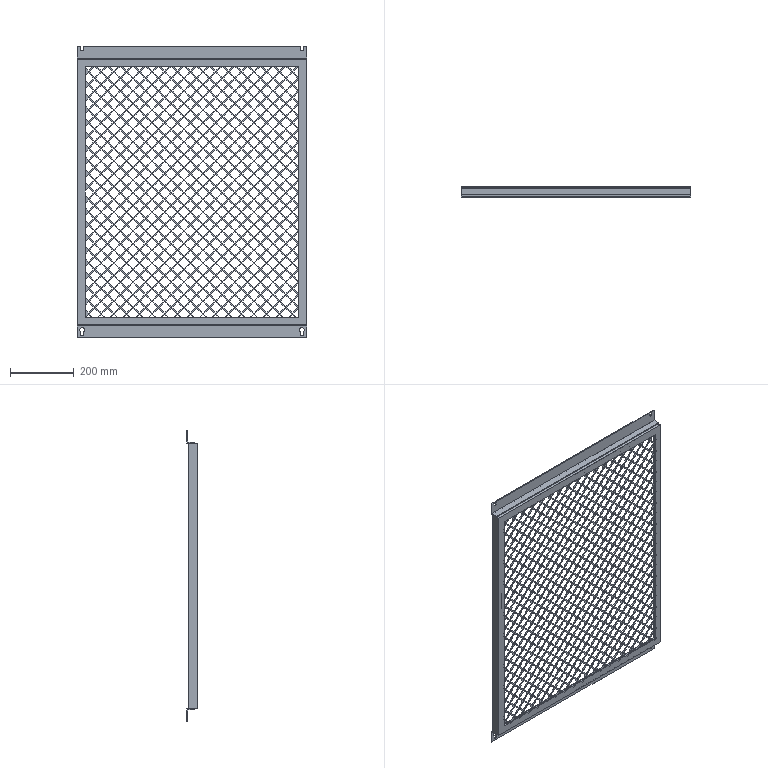Part | STEP file | OP10-007_rear cover (L) | 4 solids | 3032 faces | volume 1150842 mm3 | plane 3024 | cylinder 8 | commonest cylinder face diameters 8 x4 15 x4